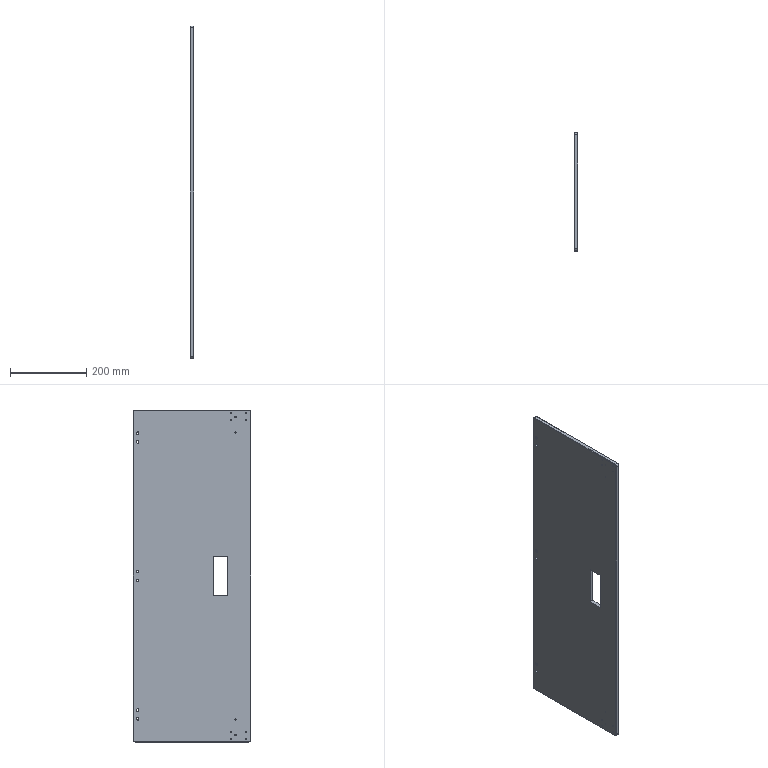Part | NX | 1 solid | 48 faces | box 10 x 308 x 869 mm | volume 2633126 mm3 | cylinder 22 | plane 18 | cone 8 | commonest cylinder face diameters 2.5 x8 6.5 x6 3.3 x4 10 x4
STEP:
#1=CARTESIAN_POINT('',(10.,-268.,-377.35));
#2=VERTEX_POINT('',#1);
#3=CARTESIAN_POINT('',(10.,-268.,-375.7));
#4=DIRECTION('',(1.,0.,0.));
#5=DIRECTION('',(0.,0.,-1.));
#6=AXIS2_PLACEMENT_3D('',#3,#4,#5);
#7=CIRCLE('',#6,1.65);
#8=EDGE_CURVE('',#2,#2,#7,.T.);
#9=ORIENTED_EDGE('',*,*,#8,.F.);
#10=EDGE_LOOP('',(#9));
#11=FACE_BOUND('',#10,.T.);
#12=CARTESIAN_POINT('',(10.,-268.,414.05));
#13=VERTEX_POINT('',#12);
#14=CARTESIAN_POINT('',(10.,-268.,415.7));
#15=DIRECTION('',(1.,0.,0.));
#16=DIRECTION('',(0.,0.,-1.));
#17=AXIS2_PLACEMENT_3D('',#14,#15,#16);
#18=CIRCLE('',#17,1.65);
#19=EDGE_CURVE('',#13,#13,#18,.T.);
#20=ORIENTED_EDGE('',*,*,#19,.F.);
#21=EDGE_LOOP('',(#20));
#22=FACE_BOUND('',#21,.T.);
#23=CARTESIAN_POINT('',(10.,-268.,374.05));
#24=VERTEX_POINT('',#23);
#25=CARTESIAN_POINT('',(10.,-268.,375.7));
#26=DIRECTION('',(1.,0.,0.));
#27=DIRECTION('',(0.,0.,-1.));
#28=AXIS2_PLACEMENT_3D('',#25,#26,#27);
#29=CIRCLE('',#28,1.65);
#30=EDGE_CURVE('',#24,#24,#29,.T.);
#31=ORIENTED_EDGE('',*,*,#30,.F.);
#32=EDGE_LOOP('',(#31));
#33=FACE_BOUND('',#32,.T.);
#34=CARTESIAN_POINT('',(10.,-256.,407.25));
#35=VERTEX_POINT('',#34);
#36=CARTESIAN_POINT('',(10.,-256.,408.5));
#37=DIRECTION('',(1.,0.,0.));
#38=DIRECTION('',(0.,0.,-1.));
#39=AXIS2_PLACEMENT_3D('',#36,#37,#38);
#40=CIRCLE('',#39,1.25);
#41=EDGE_CURVE('',#35,#35,#40,.T.);
#42=ORIENTED_EDGE('',*,*,#41,.F.);
#43=EDGE_LOOP('',(#42));
#44=FACE_BOUND('',#43,.T.);
#45=CARTESIAN_POINT('',(10.,-296.,407.25));
#46=VERTEX_POINT('',#45);
#47=CARTESIAN_POINT('',(10.,-296.,408.5));
#48=DIRECTION('',(1.,0.,0.));
#49=DIRECTION('',(0.,0.,-1.));
#50=AXIS2_PLACEMENT_3D('',#47,#48,#49);
#51=CIRCLE('',#50,1.25);
#52=EDGE_CURVE('',#46,#46,#51,.T.);
#53=ORIENTED_EDGE('',*,*,#52,.F.);
#54=EDGE_LOOP('',(#53));
#55=FACE_BOUND('',#54,.T.);
#56=CARTESIAN_POINT('',(10.,-296.,425.25));
#57=VERTEX_POINT('',#56);
#58=CARTESIAN_POINT('',(10.,-296.,426.5));
#59=DIRECTION('',(1.,0.,0.));
#60=DIRECTION('',(0.,0.,-1.));
#61=AXIS2_PLACEMENT_3D('',#58,#59,#60);
#62=CIRCLE('',#61,1.25);
#63=EDGE_CURVE('',#57,#57,#62,.T.);
#64=ORIENTED_EDGE('',*,*,#63,.F.);
#65=EDGE_LOOP('',(#64));
#66=FACE_BOUND('',#65,.T.);
#67=CARTESIAN_POINT('',(10.,-256.,425.25));
#68=VERTEX_POINT('',#67);
#69=CARTESIAN_POINT('',(10.,-256.,426.5));
#70=DIRECTION('',(1.,0.,0.));
#71=DIRECTION('',(0.,0.,-1.));
#72=AXIS2_PLACEMENT_3D('',#69,#70,#71);
#73=CIRCLE('',#72,1.25);
#74=EDGE_CURVE('',#68,#68,#73,.T.);
#75=ORIENTED_EDGE('',*,*,#74,.F.);
#76=EDGE_LOOP('',(#75));
#77=FACE_BOUND('',#76,.T.);
#78=CARTESIAN_POINT('',(10.,-256.,-427.75));
#79=VERTEX_POINT('',#78);
#80=CARTESIAN_POINT('',(10.,-256.,-426.5));
#81=DIRECTION('',(1.,0.,0.));
#82=DIRECTION('',(0.,0.,-1.));
#83=AXIS2_PLACEMENT_3D('',#80,#81,#82);
#84=CIRCLE('',#83,1.25);
#85=EDGE_CURVE('',#79,#79,#84,.T.);
#86=ORIENTED_EDGE('',*,*,#85,.F.);
#87=EDGE_LOOP('',(#86));
#88=FACE_BOUND('',#87,.T.);
#89=CARTESIAN_POINT('',(10.,-296.,-427.75));
#90=VERTEX_POINT('',#89);
#91=CARTESIAN_POINT('',(10.,-296.,-426.5));
#92=DIRECTION('',(1.,0.,0.));
#93=DIRECTION('',(0.,0.,-1.));
#94=AXIS2_PLACEMENT_3D('',#91,#92,#93);
#95=CIRCLE('',#94,1.25);
#96=EDGE_CURVE('',#90,#90,#95,.T.);
#97=ORIENTED_EDGE('',*,*,#96,.F.);
#98=EDGE_LOOP('',(#97));
#99=FACE_BOUND('',#98,.T.);
#100=CARTESIAN_POINT('',(10.,-296.,-409.75));
#101=VERTEX_POINT('',#100);
#102=CARTESIAN_POINT('',(10.,-296.,-408.5));
#103=DIRECTION('',(1.,0.,0.));
#104=DIRECTION('',(0.,0.,-1.));
#105=AXIS2_PLACEMENT_3D('',#102,#103,#104);
#106=CIRCLE('',#105,1.25);
#107=EDGE_CURVE('',#101,#101,#106,.T.);
#108=ORIENTED_EDGE('',*,*,#107,.F.);
#109=EDGE_LOOP('',(#108));
#110=FACE_BOUND('',#109,.T.);
#111=CARTESIAN_POINT('',(10.,-256.,-409.75));
#112=VERTEX_POINT('',#111);
#113=CARTESIAN_POINT('',(10.,-256.,-408.5));
#114=DIRECTION('',(1.,0.,0.));
#115=DIRECTION('',(0.,0.,-1.));
#116=AXIS2_PLACEMENT_3D('',#113,#114,#115);
#117=CIRCLE('',#116,1.25);
#118=EDGE_CURVE('',#112,#112,#117,.T.);
#119=ORIENTED_EDGE('',*,*,#118,.F.);
#120=EDGE_LOOP('',(#119));
#121=FACE_BOUND('',#120,.T.);
#122=CARTESIAN_POINT('',(10.,-5.,-433.5));
#123=VERTEX_POINT('',#122);
#124=CARTESIAN_POINT('',(10.,-1.,-429.5));
#125=VERTEX_POINT('',#124);
#126=CARTESIAN_POINT('',(10.,-5.,-429.5));
#127=DIRECTION('',(-1.,0.,0.));
#128=DIRECTION('',(0.,-1.,0.));
#129=AXIS2_PLACEMENT_3D('',#126,#127,#128);
#130=CIRCLE('',#129,4.);
#131=EDGE_CURVE('',#123,#125,#130,.F.);
#132=ORIENTED_EDGE('',*,*,#131,.T.);
#133=CARTESIAN_POINT('',(10.,-1.,429.5));
#134=VERTEX_POINT('',#133);
#135=CARTESIAN_POINT('',(10.,-1.,434.5));
#136=DIRECTION('',(0.,0.,1.));
#137=VECTOR('',#136,1000.);
#138=LINE('',#135,#137);
#139=EDGE_CURVE('',#125,#134,#138,.T.);
#140=ORIENTED_EDGE('',*,*,#139,.T.);
#141=CARTESIAN_POINT('',(10.,-5.,433.5));
#142=VERTEX_POINT('',#141);
#143=CARTESIAN_POINT('',(10.,-5.,429.5));
#144=DIRECTION('',(-1.,0.,0.));
#145=DIRECTION('',(0.,-1.,0.));
#146=AXIS2_PLACEMENT_3D('',#143,#144,#145);
#147=CIRCLE('',#146,4.);
#148=EDGE_CURVE('',#134,#142,#147,.F.);
#149=ORIENTED_EDGE('',*,*,#148,.T.);
#150=CARTESIAN_POINT('',(10.,-303.,433.5));
#151=VERTEX_POINT('',#150);
#152=CARTESIAN_POINT('',(10.,0.,433.5));
#153=DIRECTION('',(0.,-1.,0.));
#154=VECTOR('',#153,1000.);
#155=LINE('',#152,#154);
#156=EDGE_CURVE('',#142,#151,#155,.T.);
#157=ORIENTED_EDGE('',*,*,#156,.T.);
#158=CARTESIAN_POINT('',(10.,-307.,429.5));
#159=VERTEX_POINT('',#158);
#160=CARTESIAN_POINT('',(10.,-303.,429.5));
#161=DIRECTION('',(-1.,0.,0.));
#162=DIRECTION('',(0.,-1.,0.));
#163=AXIS2_PLACEMENT_3D('',#160,#161,#162);
#164=CIRCLE('',#163,4.);
#165=EDGE_CURVE('',#151,#159,#164,.F.);
#166=ORIENTED_EDGE('',*,*,#165,.T.);
#167=CARTESIAN_POINT('',(10.,-307.,-429.5));
#168=VERTEX_POINT('',#167);
#169=CARTESIAN_POINT('',(10.,-307.,434.5));
#170=DIRECTION('',(0.,0.,-1.));
#171=VECTOR('',#170,1000.);
#172=LINE('',#169,#171);
#173=EDGE_CURVE('',#159,#168,#172,.T.);
#174=ORIENTED_EDGE('',*,*,#173,.T.);
#175=CARTESIAN_POINT('',(10.,-303.,-433.5));
#176=VERTEX_POINT('',#175);
#177=CARTESIAN_POINT('',(10.,-303.,-429.5));
#178=DIRECTION('',(-1.,0.,0.));
#179=DIRECTION('',(0.,-1.,0.));
#180=AXIS2_PLACEMENT_3D('',#177,#178,#179);
#181=CIRCLE('',#180,4.);
#182=EDGE_CURVE('',#168,#176,#181,.F.);
#183=ORIENTED_EDGE('',*,*,#182,.T.);
#184=CARTESIAN_POINT('',(10.,-5.,-433.5));
#185=DIRECTION('',(0.,1.,0.));
#186=VECTOR('',#185,1000.);
#187=LINE('',#184,#186);
#188=EDGE_CURVE('',#176,#123,#187,.T.);
#189=ORIENTED_EDGE('',*,*,#188,.T.);
#190=EDGE_LOOP('',(#132,#140,#149,#157,#166,#174,#183,#189));
#191=FACE_BOUND('',#190,.T.);
#192=CARTESIAN_POINT('',(10.,-12.,-377.25));
#193=VERTEX_POINT('',#192);
#194=CARTESIAN_POINT('',(10.,-12.,-374.));
#195=DIRECTION('',(1.,0.,0.));
#196=DIRECTION('',(0.,0.,-1.));
#197=AXIS2_PLACEMENT_3D('',#194,#195,#196);
#198=CIRCLE('',#197,3.25);
#199=EDGE_CURVE('',#193,#193,#198,.T.);
#200=ORIENTED_EDGE('',*,*,#199,.F.);
#201=EDGE_LOOP('',(#200));
#202=FACE_BOUND('',#201,.T.);
#203=CARTESIAN_POINT('',(10.,-12.,-354.25));
#204=VERTEX_POINT('',#203);
#205=CARTESIAN_POINT('',(10.,-12.,-351.));
#206=DIRECTION('',(1.,0.,0.));
#207=DIRECTION('',(0.,0.,-1.));
#208=AXIS2_PLACEMENT_3D('',#205,#206,#207);
#209=CIRCLE('',#208,3.25);
#210=EDGE_CURVE('',#204,#204,#209,.T.);
#211=ORIENTED_EDGE('',*,*,#210,.F.);
#212=EDGE_LOOP('',(#211));
#213=FACE_BOUND('',#212,.T.);
#214=CARTESIAN_POINT('',(10.,-12.,347.75));
#215=VERTEX_POINT('',#214);
#216=CARTESIAN_POINT('',(10.,-12.,351.));
#217=DIRECTION('',(1.,0.,0.));
#218=DIRECTION('',(0.,0.,-1.));
#219=AXIS2_PLACEMENT_3D('',#216,#217,#218);
#220=CIRCLE('',#219,3.25);
#221=EDGE_CURVE('',#215,#215,#220,.T.);
#222=ORIENTED_EDGE('',*,*,#221,.F.);
#223=EDGE_LOOP('',(#222));
#224=FACE_BOUND('',#223,.T.);
#225=CARTESIAN_POINT('',(10.,-12.,370.75));
#226=VERTEX_POINT('',#225);
#227=CARTESIAN_POINT('',(10.,-12.,374.));
#228=DIRECTION('',(1.,0.,0.));
#229=DIRECTION('',(0.,0.,-1.));
#230=AXIS2_PLACEMENT_3D('',#227,#228,#229);
#231=CIRCLE('',#230,3.25);
#232=EDGE_CURVE('',#226,#226,#231,.T.);
#233=ORIENTED_EDGE('',*,*,#232,.F.);
#234=EDGE_LOOP('',(#233));
#235=FACE_BOUND('',#234,.T.);
#236=CARTESIAN_POINT('',(10.,-12.,8.25));
#237=VERTEX_POINT('',#236);
#238=CARTESIAN_POINT('',(10.,-12.,11.5));
#239=DIRECTION('',(1.,0.,0.));
#240=DIRECTION('',(0.,0.,-1.));
#241=AXIS2_PLACEMENT_3D('',#238,#239,#240);
#242=CIRCLE('',#241,3.25);
#243=EDGE_CURVE('',#237,#237,#242,.T.);
#244=ORIENTED_EDGE('',*,*,#243,.F.);
#245=EDGE_LOOP('',(#244));
#246=FACE_BOUND('',#245,.T.);
#247=CARTESIAN_POINT('',(10.,-12.,-14.75));
#248=VERTEX_POINT('',#247);
#249=CARTESIAN_POINT('',(10.,-12.,-11.5));
#250=DIRECTION('',(1.,0.,0.));
#251=DIRECTION('',(0.,0.,-1.));
#252=AXIS2_PLACEMENT_3D('',#249,#250,#251);
#253=CIRCLE('',#252,3.25);
#254=EDGE_CURVE('',#248,#248,#253,.T.);
#255=ORIENTED_EDGE('',*,*,#254,.F.);
#256=EDGE_LOOP('',(#255));
#257=FACE_BOUND('',#256,.T.);
#258=CARTESIAN_POINT('',(10.,-211.,-51.5));
#259=VERTEX_POINT('',#258);
#260=CARTESIAN_POINT('',(10.,-211.,51.5));
#261=VERTEX_POINT('',#260);
#262=CARTESIAN_POINT('',(10.,-211.,51.5));
#263=DIRECTION('',(0.,0.,1.));
#264=VECTOR('',#263,1000.);
#265=LINE('',#262,#264);
#266=EDGE_CURVE('',#259,#261,#265,.T.);
#267=ORIENTED_EDGE('',*,*,#266,.F.);
#268=CARTESIAN_POINT('',(10.,-248.,-51.5));
#269=VERTEX_POINT('',#268);
#270=CARTESIAN_POINT('',(10.,-211.,-51.5));
#271=DIRECTION('',(0.,1.,0.));
#272=VECTOR('',#271,1000.);
#273=LINE('',#270,#272);
#274=EDGE_CURVE('',#269,#259,#273,.T.);
#275=ORIENTED_EDGE('',*,*,#274,.F.);
#276=CARTESIAN_POINT('',(10.,-248.,51.5));
#277=VERTEX_POINT('',#276);
#278=CARTESIAN_POINT('',(10.,-248.,51.5));
#279=DIRECTION('',(0.,0.,-1.));
#280=VECTOR('',#279,1000.);
#281=LINE('',#278,#280);
#282=EDGE_CURVE('',#277,#269,#281,.T.);
#283=ORIENTED_EDGE('',*,*,#282,.F.);
#284=CARTESIAN_POINT('',(10.,-211.,51.5));
#285=DIRECTION('',(0.,-1.,0.));
#286=VECTOR('',#285,1000.);
#287=LINE('',#284,#286);
#288=EDGE_CURVE('',#261,#277,#287,.T.);
#289=ORIENTED_EDGE('',*,*,#288,.F.);
#290=EDGE_LOOP('',(#267,#275,#283,#289));
#291=FACE_BOUND('',#290,.T.);
#292=CARTESIAN_POINT('',(10.,-268.,-417.35));
#293=VERTEX_POINT('',#292);
#294=CARTESIAN_POINT('',(10.,-268.,-415.7));
#295=DIRECTION('',(1.,0.,0.));
#296=DIRECTION('',(0.,0.,-1.));
#297=AXIS2_PLACEMENT_3D('',#294,#295,#296);
#298=CIRCLE('',#297,1.65);
#299=EDGE_CURVE('',#293,#293,#298,.T.);
#300=ORIENTED_EDGE('',*,*,#299,.F.);
#301=EDGE_LOOP('',(#300));
#302=FACE_BOUND('',#301,.T.);
#303=CARTESIAN_POINT('',(10.,0.,434.5));
#304=DIRECTION('',(-1.,0.,0.));
#305=DIRECTION('',(0.,-1.,0.));
#306=AXIS2_PLACEMENT_3D('',#303,#304,#305);
#307=PLANE('',#306);
#308=ADVANCED_FACE('',(#11,#22,#33,#44,#55,#66,#77,#88,#99,#110,#121,#191,#202,#213,#224,#235,#246,#257,#291,#302),#307,.F.);
#309=CARTESIAN_POINT('',(0.,-268.,-417.35));
#310=VERTEX_POINT('',#309);
#311=CARTESIAN_POINT('',(0.,-268.,-415.7));
#312=DIRECTION('',(1.,0.,0.));
#313=DIRECTION('',(0.,0.,-1.));
#314=AXIS2_PLACEMENT_3D('',#311,#312,#313);
#315=CIRCLE('',#314,1.65);
#316=EDGE_CURVE('',#310,#310,#315,.T.);
#317=ORIENTED_EDGE('',*,*,#316,.T.);
#318=EDGE_LOOP('',(#317));
#319=FACE_BOUND('',#318,.T.);
#320=CARTESIAN_POINT('',(0.,-268.,-377.35));
#321=VERTEX_POINT('',#320);
#322=CARTESIAN_POINT('',(0.,-268.,-375.7));
#323=DIRECTION('',(1.,0.,0.));
#324=DIRECTION('',(0.,0.,-1.));
#325=AXIS2_PLACEMENT_3D('',#322,#323,#324);
#326=CIRCLE('',#325,1.65);
#327=EDGE_CURVE('',#321,#321,#326,.T.);
#328=ORIENTED_EDGE('',*,*,#327,.T.);
#329=EDGE_LOOP('',(#328));
#330=FACE_BOUND('',#329,.T.);
#331=CARTESIAN_POINT('',(0.,-268.,414.05));
#332=VERTEX_POINT('',#331);
#333=CARTESIAN_POINT('',(0.,-268.,415.7));
#334=DIRECTION('',(1.,0.,0.));
#335=DIRECTION('',(0.,0.,-1.));
#336=AXIS2_PLACEMENT_3D('',#333,#334,#335);
#337=CIRCLE('',#336,1.65);
#338=EDGE_CURVE('',#332,#332,#337,.T.);
#339=ORIENTED_EDGE('',*,*,#338,.T.);
#340=EDGE_LOOP('',(#339));
#341=FACE_BOUND('',#340,.T.);
#342=CARTESIAN_POINT('',(0.,-268.,374.05));
#343=VERTEX_POINT('',#342);
#344=CARTESIAN_POINT('',(0.,-268.,375.7));
#345=DIRECTION('',(1.,0.,0.));
#346=DIRECTION('',(0.,0.,-1.));
#347=AXIS2_PLACEMENT_3D('',#344,#345,#346);
#348=CIRCLE('',#347,1.65);
#349=EDGE_CURVE('',#343,#343,#348,.T.);
#350=ORIENTED_EDGE('',*,*,#349,.T.);
#351=EDGE_LOOP('',(#350));
#352=FACE_BOUND('',#351,.T.);
#353=CARTESIAN_POINT('',(0.,-256.,407.25));
#354=VERTEX_POINT('',#353);
#355=CARTESIAN_POINT('',(0.,-256.,408.5));
#356=DIRECTION('',(1.,0.,0.));
#357=DIRECTION('',(0.,0.,-1.));
#358=AXIS2_PLACEMENT_3D('',#355,#356,#357);
#359=CIRCLE('',#358,1.25);
#360=EDGE_CURVE('',#354,#354,#359,.T.);
#361=ORIENTED_EDGE('',*,*,#360,.T.);
#362=EDGE_LOOP('',(#361));
#363=FACE_BOUND('',#362,.T.);
#364=CARTESIAN_POINT('',(0.,-296.,407.25));
#365=VERTEX_POINT('',#364);
#366=CARTESIAN_POINT('',(0.,-296.,408.5));
#367=DIRECTION('',(1.,0.,0.));
#368=DIRECTION('',(0.,0.,-1.));
#369=AXIS2_PLACEMENT_3D('',#366,#367,#368);
#370=CIRCLE('',#369,1.25);
#371=EDGE_CURVE('',#365,#365,#370,.T.);
#372=ORIENTED_EDGE('',*,*,#371,.T.);
#373=EDGE_LOOP('',(#372));
#374=FACE_BOUND('',#373,.T.);
#375=CARTESIAN_POINT('',(0.,-296.,425.25));
#376=VERTEX_POINT('',#375);
#377=CARTESIAN_POINT('',(0.,-296.,426.5));
#378=DIRECTION('',(1.,0.,0.));
#379=DIRECTION('',(0.,0.,-1.));
#380=AXIS2_PLACEMENT_3D('',#377,#378,#379);
#381=CIRCLE('',#380,1.25);
#382=EDGE_CURVE('',#376,#376,#381,.T.);
#383=ORIENTED_EDGE('',*,*,#382,.T.);
#384=EDGE_LOOP('',(#383));
#385=FACE_BOUND('',#384,.T.);
#386=CARTESIAN_POINT('',(0.,-256.,425.25));
#387=VERTEX_POINT('',#386);
#388=CARTESIAN_POINT('',(0.,-256.,426.5));
#389=DIRECTION('',(1.,0.,0.));
#390=DIRECTION('',(0.,0.,-1.));
#391=AXIS2_PLACEMENT_3D('',#388,#389,#390);
#392=CIRCLE('',#391,1.25);
#393=EDGE_CURVE('',#387,#387,#392,.T.);
#394=ORIENTED_EDGE('',*,*,#393,.T.);
#395=EDGE_LOOP('',(#394));
#396=FACE_BOUND('',#395,.T.);
#397=CARTESIAN_POINT('',(0.,-256.,-427.75));
#398=VERTEX_POINT('',#397);
#399=CARTESIAN_POINT('',(0.,-256.,-426.5));
#400=DIRECTION('',(1.,0.,0.));
#401=DIRECTION('',(0.,0.,-1.));
#402=AXIS2_PLACEMENT_3D('',#399,#400,#401);
#403=CIRCLE('',#402,1.25);
#404=EDGE_CURVE('',#398,#398,#403,.T.);
#405=ORIENTED_EDGE('',*,*,#404,.T.);
#406=EDGE_LOOP('',(#405));
#407=FACE_BOUND('',#406,.T.);
#408=CARTESIAN_POINT('',(0.,-296.,-427.75));
#409=VERTEX_POINT('',#408);
#410=CARTESIAN_POINT('',(0.,-296.,-426.5));
#411=DIRECTION('',(1.,0.,0.));
#412=DIRECTION('',(0.,0.,-1.));
#413=AXIS2_PLACEMENT_3D('',#410,#411,#412);
#414=CIRCLE('',#413,1.25);
#415=EDGE_CURVE('',#409,#409,#414,.T.);
#416=ORIENTED_EDGE('',*,*,#415,.T.);
#417=EDGE_LOOP('',(#416));
#418=FACE_BOUND('',#417,.T.);
#419=CARTESIAN_POINT('',(0.,-296.,-409.75));
#420=VERTEX_POINT('',#419);
#421=CARTESIAN_POINT('',(0.,-296.,-408.5));
#422=DIRECTION('',(1.,0.,0.));
#423=DIRECTION('',(0.,0.,-1.));
#424=AXIS2_PLACEMENT_3D('',#421,#422,#423);
#425=CIRCLE('',#424,1.25);
#426=EDGE_CURVE('',#420,#420,#425,.T.);
#427=ORIENTED_EDGE('',*,*,#426,.T.);
#428=EDGE_LOOP('',(#427));
#429=FACE_BOUND('',#428,.T.);
#430=CARTESIAN_POINT('',(0.,-256.,-409.75));
#431=VERTEX_POINT('',#430);
#432=CARTESIAN_POINT('',(0.,-256.,-408.5));
#433=DIRECTION('',(1.,0.,0.));
#434=DIRECTION('',(0.,0.,-1.));
#435=AXIS2_PLACEMENT_3D('',#432,#433,#434);
#436=CIRCLE('',#435,1.25);
#437=EDGE_CURVE('',#431,#431,#436,.T.);
#438=ORIENTED_EDGE('',*,*,#437,.T.);
#439=EDGE_LOOP('',(#438));
#440=FACE_BOUND('',#439,.T.);
#441=CARTESIAN_POINT('',(0.,-5.,433.5));
#442=VERTEX_POINT('',#441);
#443=CARTESIAN_POINT('',(0.,-1.,429.5));
#444=VERTEX_POINT('',#443);
#445=CARTESIAN_POINT('',(0.,-5.,429.5));
#446=DIRECTION('',(1.,0.,0.));
#447=DIRECTION('',(0.,0.,-1.));
#448=AXIS2_PLACEMENT_3D('',#445,#446,#447);
#449=CIRCLE('',#448,4.);
#450=EDGE_CURVE('',#442,#444,#449,.F.);
#451=ORIENTED_EDGE('',*,*,#450,.T.);
#452=CARTESIAN_POINT('',(0.,-1.,-429.5));
#453=VERTEX_POINT('',#452);
#454=CARTESIAN_POINT('',(0.,-1.,434.5));
#455=DIRECTION('',(0.,0.,-1.));
#456=VECTOR('',#455,1000.);
#457=LINE('',#454,#456);
#458=EDGE_CURVE('',#444,#453,#457,.T.);
#459=ORIENTED_EDGE('',*,*,#458,.T.);
#460=CARTESIAN_POINT('',(0.,-5.,-433.5));
#461=VERTEX_POINT('',#460);
#462=CARTESIAN_POINT('',(0.,-5.,-429.5));
#463=DIRECTION('',(1.,0.,0.));
#464=DIRECTION('',(0.,0.,-1.));
#465=AXIS2_PLACEMENT_3D('',#462,#463,#464);
#466=CIRCLE('',#465,4.);
#467=EDGE_CURVE('',#453,#461,#466,.F.);
#468=ORIENTED_EDGE('',*,*,#467,.T.);
#469=CARTESIAN_POINT('',(0.,-303.,-433.5));
#470=VERTEX_POINT('',#469);
#471=CARTESIAN_POINT('',(0.,-303.,-433.5));
#472=DIRECTION('',(0.,-1.,0.));
#473=VECTOR('',#472,1000.);
#474=LINE('',#471,#473);
#475=EDGE_CURVE('',#461,#470,#474,.T.);
#476=ORIENTED_EDGE('',*,*,#475,.T.);
#477=CARTESIAN_POINT('',(0.,-307.,-429.5));
#478=VERTEX_POINT('',#477);
#479=CARTESIAN_POINT('',(0.,-303.,-429.5));
#480=DIRECTION('',(1.,0.,0.));
#481=DIRECTION('',(0.,0.,-1.));
#482=AXIS2_PLACEMENT_3D('',#479,#480,#481);
#483=CIRCLE('',#482,4.);
#484=EDGE_CURVE('',#470,#478,#483,.F.);
#485=ORIENTED_EDGE('',*,*,#484,.T.);
#486=CARTESIAN_POINT('',(0.,-307.,429.5));
#487=VERTEX_POINT('',#486);
#488=CARTESIAN_POINT('',(0.,-307.,434.5));
#489=DIRECTION('',(0.,0.,1.));
#490=VECTOR('',#489,1000.);
#491=LINE('',#488,#490);
#492=EDGE_CURVE('',#478,#487,#491,.T.);
#493=ORIENTED_EDGE('',*,*,#492,.T.);
#494=CARTESIAN_POINT('',(0.,-303.,433.5));
#495=VERTEX_POINT('',#494);
#496=CARTESIAN_POINT('',(0.,-303.,429.5));
#497=DIRECTION('',(1.,0.,0.));
#498=DIRECTION('',(0.,0.,-1.));
#499=AXIS2_PLACEMENT_3D('',#496,#497,#498);
#500=CIRCLE('',#499,4.);
#501=EDGE_CURVE('',#487,#495,#500,.F.);
#502=ORIENTED_EDGE('',*,*,#501,.T.);
#503=CARTESIAN_POINT('',(0.,-308.,433.5));
#504=DIRECTION('',(0.,1.,0.));
#505=VECTOR('',#504,1000.);
#506=LINE('',#503,#505);
#507=EDGE_CURVE('',#495,#442,#506,.T.);
#508=ORIENTED_EDGE('',*,*,#507,.T.);
#509=EDGE_LOOP('',(#451,#459,#468,#476,#485,#493,#502,#508));
#510=FACE_BOUND('',#509,.T.);
#511=CARTESIAN_POINT('',(0.,-12.,-377.25));
#512=VERTEX_POINT('',#511);
#513=CARTESIAN_POINT('',(0.,-12.,-374.));
#514=DIRECTION('',(1.,0.,0.));
#515=DIRECTION('',(0.,0.,-1.));
#516=AXIS2_PLACEMENT_3D('',#513,#514,#515);
#517=CIRCLE('',#516,3.25);
#518=EDGE_CURVE('',#512,#512,#517,.T.);
#519=ORIENTED_EDGE('',*,*,#518,.T.);
#520=EDGE_LOOP('',(#519));
#521=FACE_BOUND('',#520,.T.);
#522=CARTESIAN_POINT('',(0.,-12.,-354.25));
#523=VERTEX_POINT('',#522);
#524=CARTESIAN_POINT('',(0.,-12.,-351.));
#525=DIRECTION('',(1.,0.,0.));
#526=DIRECTION('',(0.,0.,-1.));
#527=AXIS2_PLACEMENT_3D('',#524,#525,#526);
#528=CIRCLE('',#527,3.25);
#529=EDGE_CURVE('',#523,#523,#528,.T.);
#530=ORIENTED_EDGE('',*,*,#529,.T.);
#531=EDGE_LOOP('',(#530));
#532=FACE_BOUND('',#531,.T.);
#533=CARTESIAN_POINT('',(0.,-12.,347.75));
#534=VERTEX_POINT('',#533);
#535=CARTESIAN_POINT('',(0.,-12.,351.));
#536=DIRECTION('',(1.,0.,0.));
#537=DIRECTION('',(0.,0.,-1.));
#538=AXIS2_PLACEMENT_3D('',#535,#536,#537);
#539=CIRCLE('',#538,3.25);
#540=EDGE_CURVE('',#534,#534,#539,.T.);
#541=ORIENTED_EDGE('',*,*,#540,.T.);
#542=EDGE_LOOP('',(#541));
#543=FACE_BOUND('',#542,.T.);
#544=CARTESIAN_POINT('',(0.,-12.,370.75));
#545=VERTEX_POINT('',#544);
#546=CARTESIAN_POINT('',(0.,-12.,374.));
#547=DIRECTION('',(1.,0.,0.));
#548=DIRECTION('',(0.,0.,-1.));
#549=AXIS2_PLACEMENT_3D('',#546,#547,#548);
#550=CIRCLE('',#549,3.25);
#551=EDGE_CURVE('',#545,#545,#550,.T.);
#552=ORIENTED_EDGE('',*,*,#551,.T.);
#553=EDGE_LOOP('',(#552));
#554=FACE_BOUND('',#553,.T.);
#555=CARTESIAN_POINT('',(0.,-12.,8.25));
#556=VERTEX_POINT('',#555);
#557=CARTESIAN_POINT('',(0.,-12.,11.5));
#558=DIRECTION('',(1.,0.,0.));
#559=DIRECTION('',(0.,0.,-1.));
#560=AXIS2_PLACEMENT_3D('',#557,#558,#559);
#561=CIRCLE('',#560,3.25);
#562=EDGE_CURVE('',#556,#556,#561,.T.);
#563=ORIENTED_EDGE('',*,*,#562,.T.);
#564=EDGE_LOOP('',(#563));
#565=FACE_BOUND('',#564,.T.);
#566=CARTESIAN_POINT('',(0.,-12.,-14.75));
#567=VERTEX_POINT('',#566);
#568=CARTESIAN_POINT('',(0.,-12.,-11.5));
#569=DIRECTION('',(1.,0.,0.));
#570=DIRECTION('',(0.,0.,-1.));
#571=AXIS2_PLACEMENT_3D('',#568,#569,#570);
#572=CIRCLE('',#571,3.25);
#573=EDGE_CURVE('',#567,#567,#572,.T.);
#574=ORIENTED_EDGE('',*,*,#573,.T.);
#575=EDGE_LOOP('',(#574));
#576=FACE_BOUND('',#575,.T.);
#577=CARTESIAN_POINT('',(0.,-248.,51.5));
#578=VERTEX_POINT('',#577);
#579=CARTESIAN_POINT('',(0.,-248.,-51.5));
#580=VERTEX_POINT('',#579);
#581=CARTESIAN_POINT('',(0.,-248.,51.5));
#582=DIRECTION('',(0.,0.,-1.));
#583=VECTOR('',#582,1000.);
#584=LINE('',#581,#583);
#585=EDGE_CURVE('',#578,#580,#584,.T.);
#586=ORIENTED_EDGE('',*,*,#585,.T.);
#587=CARTESIAN_POINT('',(0.,-211.,-51.5));
#588=VERTEX_POINT('',#587);
#589=CARTESIAN_POINT('',(0.,-211.,-51.5));
#590=DIRECTION('',(0.,1.,0.));
#591=VECTOR('',#590,1000.);
#592=LINE('',#589,#591);
#593=EDGE_CURVE('',#580,#588,#592,.T.);
#594=ORIENTED_EDGE('',*,*,#593,.T.);
#595=CARTESIAN_POINT('',(0.,-211.,51.5));
#596=VERTEX_POINT('',#595);
#597=CARTESIAN_POINT('',(0.,-211.,51.5));
#598=DIRECTION('',(0.,0.,1.));
#599=VECTOR('',#598,1000.);
#600=LINE('',#597,#599);
#601=EDGE_CURVE('',#588,#596,#600,.T.);
#602=ORIENTED_EDGE('',*,*,#601,.T.);
#603=CARTESIAN_POINT('',(0.,-211.,51.5));
#604=DIRECTION('',(0.,-1.,0.));
#605=VECTOR('',#604,1000.);
#606=LINE('',#603,#605);
#607=EDGE_CURVE('',#596,#578,#606,.T.);
#608=ORIENTED_EDGE('',*,*,#607,.T.);
#609=EDGE_LOOP('',(#586,#594,#602,#608));
#610=FACE_BOUND('',#609,.T.);
#611=CARTESIAN_POINT('',(0.,-308.,434.5));
#612=DIRECTION('',(1.,0.,0.));
#613=DIRECTION('',(0.,0.,-1.));
#614=AXIS2_PLACEMENT_3D('',#611,#612,#613);
#615=PLANE('',#614);
#616=ADVANCED_FACE('',(#319,#330,#341,#352,#363,#374,#385,#396,#407,#418,#429,#440,#510,#521,#532,#543,#554,#565,#576,#610),#615,.F.);
#617=CARTESIAN_POINT('',(1.,-308.,-429.5));
#618=VERTEX_POINT('',#617);
#619=CARTESIAN_POINT('',(9.,-308.,-429.5));
#620=VERTEX_POINT('',#619);
#621=CARTESIAN_POINT('',(10.,-308.,-429.5));
#622=DIRECTION('',(1.,0.,0.));
#623=VECTOR('',#622,1000.);
#624=LINE('',#621,#623);
#625=EDGE_CURVE('',#618,#620,#624,.T.);
#626=ORIENTED_EDGE('',*,*,#625,.T.);
#627=CARTESIAN_POINT('',(9.,-308.,429.5));
#628=VERTEX_POINT('',#627);
#629=CARTESIAN_POINT('',(9.,-308.,434.5));
#630=DIRECTION('',(0.,0.,1.));
#631=VECTOR('',#630,1000.);
#632=LINE('',#629,#631);
#633=EDGE_CURVE('',#620,#628,#632,.T.);
#634=ORIENTED_EDGE('',*,*,#633,.T.);
#635=CARTESIAN_POINT('',(1.,-308.,429.5));
#636=VERTEX_POINT('',#635);
#637=CARTESIAN_POINT('',(10.,-308.,429.5));
#638=DIRECTION('',(1.,0.,0.));
#639=VECTOR('',#638,1000.);
#640=LINE('',#637,#639);
#641=EDGE_CURVE('',#628,#636,#640,.F.);
#642=ORIENTED_EDGE('',*,*,#641,.T.);
#643=CARTESIAN_POINT('',(1.,-308.,434.5));
#644=DIRECTION('',(0.,0.,-1.));
#645=VECTOR('',#644,1000.);
#646=LINE('',#643,#645);
#647=EDGE_CURVE('',#636,#618,#646,.T.);
#648=ORIENTED_EDGE('',*,*,#647,.T.);
#649=EDGE_LOOP('',(#626,#634,#642,#648));
#650=FACE_BOUND('',#649,.T.);
#651=CARTESIAN_POINT('',(10.,-308.,434.5));
#652=DIRECTION('',(0.,1.,0.));
#653=DIRECTION('',(0.,0.,1.));
#654=AXIS2_PLACEMENT_3D('',#651,#652,#653);
#655=PLANE('',#654);
#656=ADVANCED_FACE('',(#650),#655,.F.);
#657=CARTESIAN_POINT('',(1.,0.,429.5));
#658=VERTEX_POINT('',#657);
#659=CARTESIAN_POINT('',(9.,0.,429.5));
#660=VERTEX_POINT('',#659);
#661=CARTESIAN_POINT('',(0.,0.,429.5));
#662=DIRECTION('',(-1.,0.,0.));
#663=VECTOR('',#662,1000.);
#664=LINE('',#661,#663);
#665=EDGE_CURVE('',#658,#660,#664,.F.);
#666=ORIENTED_EDGE('',*,*,#665,.T.);
#667=CARTESIAN_POINT('',(9.,0.,-429.5));
#668=VERTEX_POINT('',#667);
#669=CARTESIAN_POINT('',(9.,0.,434.5));
#670=DIRECTION('',(0.,0.,-1.));
#671=VECTOR('',#670,1000.);
#672=LINE('',#669,#671);
#673=EDGE_CURVE('',#660,#668,#672,.T.);
#674=ORIENTED_EDGE('',*,*,#673,.T.);
#675=CARTESIAN_POINT('',(1.,0.,-429.5));
#676=VERTEX_POINT('',#675);
#677=CARTESIAN_POINT('',(0.,0.,-429.5));
#678=DIRECTION('',(-1.,0.,0.));
#679=VECTOR('',#678,1000.);
#680=LINE('',#677,#679);
#681=EDGE_CURVE('',#668,#676,#680,.T.);
#682=ORIENTED_EDGE('',*,*,#681,.T.);
#683=CARTESIAN_POINT('',(1.,0.,434.5));
#684=DIRECTION('',(0.,0.,1.));
#685=VECTOR('',#684,1000.);
#686=LINE('',#683,#685);
#687=EDGE_CURVE('',#676,#658,#686,.T.);
#688=ORIENTED_EDGE('',*,*,#687,.T.);
#689=EDGE_LOOP('',(#666,#674,#682,#688));
#690=FACE_BOUND('',#689,.T.);
#691=CARTESIAN_POINT('',(0.,0.,434.5));
#692=DIRECTION('',(0.,-1.,0.));
#693=DIRECTION('',(1.,0.,0.));
#694=AXIS2_PLACEMENT_3D('',#691,#692,#693);
#695=PLANE('',#694);
#696=ADVANCED_FACE('',(#690),#695,.F.);
#697=CARTESIAN_POINT('',(1.,-303.,434.5));
#698=VERTEX_POINT('',#697);
#699=CARTESIAN_POINT('',(9.,-303.,434.5));
#700=VERTEX_POINT('',#699);
#701=CARTESIAN_POINT('',(0.,-303.,434.5));
#702=DIRECTION('',(1.,0.,0.));
#703=VECTOR('',#702,1000.);
#704=LINE('',#701,#703);
#705=EDGE_CURVE('',#698,#700,#704,.T.);
#706=ORIENTED_EDGE('',*,*,#705,.T.);
#707=CARTESIAN_POINT('',(9.,-5.,434.5));
#708=VERTEX_POINT('',#707);
#709=CARTESIAN_POINT('',(9.,0.,434.5));
#710=DIRECTION('',(0.,1.,0.));
#711=VECTOR('',#710,1000.);
#712=LINE('',#709,#711);
#713=EDGE_CURVE('',#700,#708,#712,.T.);
#714=ORIENTED_EDGE('',*,*,#713,.T.);
#715=CARTESIAN_POINT('',(1.,-5.,434.5));
#716=VERTEX_POINT('',#715);
#717=CARTESIAN_POINT('',(0.,-5.,434.5));
#718=DIRECTION('',(-1.,0.,0.));
#719=VECTOR('',#718,1000.);
#720=LINE('',#717,#719);
#721=EDGE_CURVE('',#708,#716,#720,.T.);
#722=ORIENTED_EDGE('',*,*,#721,.T.);
#723=CARTESIAN_POINT('',(1.,0.,434.5));
#724=DIRECTION('',(0.,-1.,0.));
#725=VECTOR('',#724,1000.);
#726=LINE('',#723,#725);
#727=EDGE_CURVE('',#716,#698,#726,.T.);
#728=ORIENTED_EDGE('',*,*,#727,.T.);
#729=EDGE_LOOP('',(#706,#714,#722,#728));
#730=FACE_BOUND('',#729,.T.);
#731=CARTESIAN_POINT('',(0.,0.,434.5));
#732=DIRECTION('',(0.,0.,-1.));
#733=DIRECTION('',(-1.,0.,0.));
#734=AXIS2_PLACEMENT_3D('',#731,#732,#733);
#735=PLANE('',#734);
#736=ADVANCED_FACE('',(#730),#735,.F.);
#737=CARTESIAN_POINT('',(1.,-5.,-434.5));
#738=VERTEX_POINT('',#737);
#739=CARTESIAN_POINT('',(9.,-5.,-434.5));
#740=VERTEX_POINT('',#739);
#741=CARTESIAN_POINT('',(10.,-5.,-434.5));
#742=DIRECTION('',(-1.,0.,0.));
#743=VECTOR('',#742,1000.);
#744=LINE('',#741,#743);
#745=EDGE_CURVE('',#738,#740,#744,.F.);
#746=ORIENTED_EDGE('',*,*,#745,.T.);
#747=CARTESIAN_POINT('',(9.,-303.,-434.5));
#748=VERTEX_POINT('',#747);
#749=CARTESIAN_POINT('',(9.,-303.,-434.5));
#750=DIRECTION('',(0.,-1.,0.));
#751=VECTOR('',#750,1000.);
#752=LINE('',#749,#751);
#753=EDGE_CURVE('',#740,#748,#752,.T.);
#754=ORIENTED_EDGE('',*,*,#753,.T.);
#755=CARTESIAN_POINT('',(1.,-303.,-434.5));
#756=VERTEX_POINT('',#755);
#757=CARTESIAN_POINT('',(0.,-303.,-434.5));
#758=DIRECTION('',(1.,0.,0.));
#759=VECTOR('',#758,1000.);
#760=LINE('',#757,#759);
#761=EDGE_CURVE('',#748,#756,#760,.F.);
#762=ORIENTED_EDGE('',*,*,#761,.T.);
#763=CARTESIAN_POINT('',(1.,-5.,-434.5));
#764=DIRECTION('',(0.,1.,0.));
#765=VECTOR('',#764,1000.);
#766=LINE('',#763,#765);
#767=EDGE_CURVE('',#756,#738,#766,.T.);
#768=ORIENTED_EDGE('',*,*,#767,.T.);
#769=EDGE_LOOP('',(#746,#754,#762,#768));
#770=FACE_BOUND('',#769,.T.);
#771=CARTESIAN_POINT('',(0.,0.,-434.5));
#772=DIRECTION('',(0.,0.,-1.));
#773=DIRECTION('',(-1.,0.,0.));
#774=AXIS2_PLACEMENT_3D('',#771,#772,#773);
#775=PLANE('',#774);
#776=ADVANCED_FACE('',(#770),#775,.T.);
#777=ORIENTED_EDGE('',*,*,#274,.T.);
#778=CARTESIAN_POINT('',(0.,-211.,-51.5));
#779=DIRECTION('',(1.,0.,0.));
#780=VECTOR('',#779,1000.);
#781=LINE('',#778,#780);
#782=EDGE_CURVE('',#588,#259,#781,.T.);
#783=ORIENTED_EDGE('',*,*,#782,.F.);
#784=ORIENTED_EDGE('',*,*,#593,.F.);
#785=CARTESIAN_POINT('',(0.,-248.,-51.5));
#786=DIRECTION('',(1.,0.,0.));
#787=VECTOR('',#786,1000.);
#788=LINE('',#785,#787);
#789=EDGE_CURVE('',#580,#269,#788,.T.);
#790=ORIENTED_EDGE('',*,*,#789,.T.);
#791=EDGE_LOOP('',(#777,#783,#784,#790));
#792=FACE_BOUND('',#791,.T.);
#793=CARTESIAN_POINT('',(0.,-211.,-51.5));
#794=DIRECTION('',(0.,0.,-1.));
#795=DIRECTION('',(0.,1.,0.));
#796=AXIS2_PLACEMENT_3D('',#793,#794,#795);
#797=PLANE('',#796);
#798=ADVANCED_FACE('',(#792),#797,.F.);
#799=ORIENTED_EDGE('',*,*,#282,.T.);
#800=ORIENTED_EDGE('',*,*,#789,.F.);
#801=ORIENTED_EDGE('',*,*,#585,.F.);
#802=CARTESIAN_POINT('',(0.,-248.,51.5));
#803=DIRECTION('',(1.,0.,0.));
#804=VECTOR('',#803,1000.);
#805=LINE('',#802,#804);
#806=EDGE_CURVE('',#578,#277,#805,.T.);
#807=ORIENTED_EDGE('',*,*,#806,.T.);
#808=EDGE_LOOP('',(#799,#800,#801,#807));
#809=FACE_BOUND('',#808,.T.);
#810=CARTESIAN_POINT('',(0.,-248.,51.5));
#811=DIRECTION('',(0.,-1.,0.));
#812=DIRECTION('',(1.,0.,0.));
#813=AXIS2_PLACEMENT_3D('',#810,#811,#812);
#814=PLANE('',#813);
#815=ADVANCED_FACE('',(#809),#814,.F.);
#816=ORIENTED_EDGE('',*,*,#288,.T.);
#817=ORIENTED_EDGE('',*,*,#806,.F.);
#818=ORIENTED_EDGE('',*,*,#607,.F.);
#819=CARTESIAN_POINT('',(0.,-211.,51.5));
#820=DIRECTION('',(1.,0.,0.));
#821=VECTOR('',#820,1000.);
#822=LINE('',#819,#821);
#823=EDGE_CURVE('',#596,#261,#822,.T.);
#824=ORIENTED_EDGE('',*,*,#823,.T.);
#825=EDGE_LOOP('',(#816,#817,#818,#824));
#826=FACE_BOUND('',#825,.T.);
#827=CARTESIAN_POINT('',(0.,-211.,51.5));
#828=DIRECTION('',(0.,0.,1.));
#829=DIRECTION('',(0.,-1.,0.));
#830=AXIS2_PLACEMENT_3D('',#827,#828,#829);
#831=PLANE('',#830);
#832=ADVANCED_FACE('',(#826),#831,.F.);
#833=ORIENTED_EDGE('',*,*,#266,.T.);
#834=ORIENTED_EDGE('',*,*,#823,.F.);
#835=ORIENTED_EDGE('',*,*,#601,.F.);
#836=ORIENTED_EDGE('',*,*,#782,.T.);
#837=EDGE_LOOP('',(#833,#834,#835,#836));
#838=FACE_BOUND('',#837,.T.);
#839=CARTESIAN_POINT('',(0.,-211.,51.5));
#840=DIRECTION('',(0.,1.,0.));
#841=DIRECTION('',(-1.,0.,0.));
#842=AXIS2_PLACEMENT_3D('',#839,#840,#841);
#843=PLANE('',#842);
#844=ADVANCED_FACE('',(#838),#843,.F.);
#845=ORIENTED_EDGE('',*,*,#573,.F.);
#846=EDGE_LOOP('',(#845));
#847=FACE_BOUND('',#846,.T.);
#848=ORIENTED_EDGE('',*,*,#254,.T.);
#849=EDGE_LOOP('',(#848));
#850=FACE_BOUND('',#849,.T.);
#851=CARTESIAN_POINT('',(10.,-12.,-11.5));
#852=DIRECTION('',(1.,0.,0.));
#853=DIRECTION('',(0.,0.,-1.));
#854=AXIS2_PLACEMENT_3D('',#851,#852,#853);
#855=CYLINDRICAL_SURFACE('',#854,3.25);
#856=ADVANCED_FACE('',(#847,#850),#855,.F.);
#857=ORIENTED_EDGE('',*,*,#562,.F.);
#858=EDGE_LOOP('',(#857));
#859=FACE_BOUND('',#858,.T.);
#860=ORIENTED_EDGE('',*,*,#243,.T.);
#861=EDGE_LOOP('',(#860));
#862=FACE_BOUND('',#861,.T.);
#863=CARTESIAN_POINT('',(10.,-12.,11.5));
#864=DIRECTION('',(1.,0.,0.));
#865=DIRECTION('',(0.,0.,-1.));
#866=AXIS2_PLACEMENT_3D('',#863,#864,#865);
#867=CYLINDRICAL_SURFACE('',#866,3.25);
#868=ADVANCED_FACE('',(#859,#862),#867,.F.);
#869=ORIENTED_EDGE('',*,*,#551,.F.);
#870=EDGE_LOOP('',(#869));
#871=FACE_BOUND('',#870,.T.);
#872=ORIENTED_EDGE('',*,*,#232,.T.);
#873=EDGE_LOOP('',(#872));
#874=FACE_BOUND('',#873,.T.);
#875=CARTESIAN_POINT('',(10.,-12.,374.));
#876=DIRECTION('',(1.,0.,0.));
#877=DIRECTION('',(0.,0.,-1.));
#878=AXIS2_PLACEMENT_3D('',#875,#876,#877);
#879=CYLINDRICAL_SURFACE('',#878,3.25);
#880=ADVANCED_FACE('',(#871,#874),#879,.F.);
#881=ORIENTED_EDGE('',*,*,#540,.F.);
#882=EDGE_LOOP('',(#881));
#883=FACE_BOUND('',#882,.T.);
#884=ORIENTED_EDGE('',*,*,#221,.T.);
#885=EDGE_LOOP('',(#884));
#886=FACE_BOUND('',#885,.T.);
#887=CARTESIAN_POINT('',(10.,-12.,351.));
#888=DIRECTION('',(1.,0.,0.));
#889=DIRECTION('',(0.,0.,-1.));
#890=AXIS2_PLACEMENT_3D('',#887,#888,#889);
#891=CYLINDRICAL_SURFACE('',#890,3.25);
#892=ADVANCED_FACE('',(#883,#886),#891,.F.);
#893=ORIENTED_EDGE('',*,*,#529,.F.);
#894=EDGE_LOOP('',(#893));
#895=FACE_BOUND('',#894,.T.);
#896=ORIENTED_EDGE('',*,*,#210,.T.);
#897=EDGE_LOOP('',(#896));
#898=FACE_BOUND('',#897,.T.);
#899=CARTESIAN_POINT('',(10.,-12.,-351.));
#900=DIRECTION('',(1.,0.,0.));
#901=DIRECTION('',(0.,0.,-1.));
#902=AXIS2_PLACEMENT_3D('',#899,#900,#901);
#903=CYLINDRICAL_SURFACE('',#902,3.25);
#904=ADVANCED_FACE('',(#895,#898),#903,.F.);
#905=ORIENTED_EDGE('',*,*,#518,.F.);
#906=EDGE_LOOP('',(#905));
#907=FACE_BOUND('',#906,.T.);
#908=ORIENTED_EDGE('',*,*,#199,.T.);
#909=EDGE_LOOP('',(#908));
#910=FACE_BOUND('',#909,.T.);
#911=CARTESIAN_POINT('',(10.,-12.,-374.));
#912=DIRECTION('',(1.,0.,0.));
#913=DIRECTION('',(0.,0.,-1.));
#914=AXIS2_PLACEMENT_3D('',#911,#912,#913);
#915=CYLINDRICAL_SURFACE('',#914,3.25);
#916=ADVANCED_FACE('',(#907,#910),#915,.F.);
#917=ORIENTED_EDGE('',*,*,#721,.F.);
#918=CARTESIAN_POINT('',(9.,-5.,429.5));
#919=DIRECTION('',(-1.,0.,0.));
#920=DIRECTION('',(0.,0.,1.));
#921=AXIS2_PLACEMENT_3D('',#918,#919,#920);
#922=CIRCLE('',#921,5.);
#923=EDGE_CURVE('',#708,#660,#922,.T.);
#924=ORIENTED_EDGE('',*,*,#923,.T.);
#925=ORIENTED_EDGE('',*,*,#665,.F.);
#926=CARTESIAN_POINT('',(1.,-5.,429.5));
#927=DIRECTION('',(1.,0.,0.));
#928=DIRECTION('',(0.,0.,-1.));
#929=AXIS2_PLACEMENT_3D('',#926,#927,#928);
#930=CIRCLE('',#929,5.);
#931=EDGE_CURVE('',#658,#716,#930,.T.);
#932=ORIENTED_EDGE('',*,*,#931,.T.);
#933=EDGE_LOOP('',(#917,#924,#925,#932));
#934=FACE_BOUND('',#933,.T.);
#935=CARTESIAN_POINT('',(0.,-5.,429.5));
#936=DIRECTION('',(-1.,0.,0.));
#937=DIRECTION('',(0.,-1.,0.));
#938=AXIS2_PLACEMENT_3D('',#935,#936,#937);
#939=CYLINDRICAL_SURFACE('',#938,5.);
#940=ADVANCED_FACE('',(#934),#939,.T.);
#941=ORIENTED_EDGE('',*,*,#641,.F.);
#942=CARTESIAN_POINT('',(9.,-303.,429.5));
#943=DIRECTION('',(-1.,0.,0.));
#944=DIRECTION('',(0.,0.,1.));
#945=AXIS2_PLACEMENT_3D('',#942,#943,#944);
#946=CIRCLE('',#945,5.);
#947=EDGE_CURVE('',#628,#700,#946,.T.);
#948=ORIENTED_EDGE('',*,*,#947,.T.);
#949=ORIENTED_EDGE('',*,*,#705,.F.);
#950=CARTESIAN_POINT('',(1.,-303.,429.5));
#951=DIRECTION('',(1.,0.,0.));
#952=DIRECTION('',(0.,0.,-1.));
#953=AXIS2_PLACEMENT_3D('',#950,#951,#952);
#954=CIRCLE('',#953,5.);
#955=EDGE_CURVE('',#698,#636,#954,.T.);
#956=ORIENTED_EDGE('',*,*,#955,.T.);
#957=EDGE_LOOP('',(#941,#948,#949,#956));
#958=FACE_BOUND('',#957,.T.);
#959=CARTESIAN_POINT('',(0.,-303.,429.5));
#960=DIRECTION('',(1.,0.,0.));
#961=DIRECTION('',(0.,0.,-1.));
#962=AXIS2_PLACEMENT_3D('',#959,#960,#961);
#963=CYLINDRICAL_SURFACE('',#962,5.);
#964=ADVANCED_FACE('',(#958),#963,.T.);
#965=ORIENTED_EDGE('',*,*,#681,.F.);
#966=CARTESIAN_POINT('',(9.,-5.,-429.5));
#967=DIRECTION('',(-1.,0.,0.));
#968=DIRECTION('',(0.,0.,1.));
#969=AXIS2_PLACEMENT_3D('',#966,#967,#968);
#970=CIRCLE('',#969,5.);
#971=EDGE_CURVE('',#668,#740,#970,.T.);
#972=ORIENTED_EDGE('',*,*,#971,.T.);
#973=ORIENTED_EDGE('',*,*,#745,.F.);
#974=CARTESIAN_POINT('',(1.,-5.,-429.5));
#975=DIRECTION('',(1.,0.,0.));
#976=DIRECTION('',(0.,0.,-1.));
#977=AXIS2_PLACEMENT_3D('',#974,#975,#976);
#978=CIRCLE('',#977,5.);
#979=EDGE_CURVE('',#738,#676,#978,.T.);
#980=ORIENTED_EDGE('',*,*,#979,.T.);
#981=EDGE_LOOP('',(#965,#972,#973,#980));
#982=FACE_BOUND('',#981,.T.);
#983=CARTESIAN_POINT('',(0.,-5.,-429.5));
#984=DIRECTION('',(1.,0.,0.));
#985=DIRECTION('',(0.,1.,0.));
#986=AXIS2_PLACEMENT_3D('',#983,#984,#985);
#987=CYLINDRICAL_SURFACE('',#986,5.);
#988=ADVANCED_FACE('',(#982),#987,.T.);
#989=ORIENTED_EDGE('',*,*,#761,.F.);
#990=CARTESIAN_POINT('',(9.,-303.,-429.5));
#991=DIRECTION('',(-1.,0.,0.));
#992=DIRECTION('',(0.,0.,1.));
#993=AXIS2_PLACEMENT_3D('',#990,#991,#992);
#994=CIRCLE('',#993,5.);
#995=EDGE_CURVE('',#748,#620,#994,.T.);
#996=ORIENTED_EDGE('',*,*,#995,.T.);
#997=ORIENTED_EDGE('',*,*,#625,.F.);
#998=CARTESIAN_POINT('',(1.,-303.,-429.5));
#999=DIRECTION('',(1.,0.,0.));
#1000=DIRECTION('',(0.,0.,-1.));
#1001=AXIS2_PLACEMENT_3D('',#998,#999,#1000);
#1002=CIRCLE('',#1001,5.);
#1003=EDGE_CURVE('',#618,#756,#1002,.T.);
#1004=ORIENTED_EDGE('',*,*,#1003,.T.);
#1005=EDGE_LOOP('',(#989,#996,#997,#1004));
#1006=FACE_BOUND('',#1005,.T.);
#1007=CARTESIAN_POINT('',(10.,-303.,-429.5));
#1008=DIRECTION('',(-1.,0.,0.));
#1009=DIRECTION('',(0.,0.,1.));
#1010=AXIS2_PLACEMENT_3D('',#1007,#1008,#1009);
#1011=CYLINDRICAL_SURFACE('',#1010,5.);
#1012=ADVANCED_FACE('',(#1006),#1011,.T.);
#1013=CARTESIAN_POINT('',(10.,-307.,-429.5));
#1014=DIRECTION('',(-0.7071,-0.7071,0.));
#1015=VECTOR('',#1014,1000.);
#1016=LINE('',#1013,#1015);
#1017=EDGE_CURVE('',#168,#620,#1016,.T.);
#1018=ORIENTED_EDGE('',*,*,#1017,.F.);
#1019=ORIENTED_EDGE('',*,*,#173,.F.);
#1020=CARTESIAN_POINT('',(9.,-308.,429.5));
#1021=DIRECTION('',(0.7071,0.7071,0.));
#1022=VECTOR('',#1021,1000.);
#1023=LINE('',#1020,#1022);
#1024=EDGE_CURVE('',#628,#159,#1023,.T.);
#1025=ORIENTED_EDGE('',*,*,#1024,.F.);
#1026=ORIENTED_EDGE('',*,*,#633,.F.);
#1027=EDGE_LOOP('',(#1018,#1019,#1025,#1026));
#1028=FACE_BOUND('',#1027,.T.);
#1029=CARTESIAN_POINT('',(10.,-307.,434.5));
#1030=DIRECTION('',(-0.7071,0.7071,0.));
#1031=DIRECTION('',(0.,0.,-1.));
#1032=AXIS2_PLACEMENT_3D('',#1029,#1030,#1031);
#1033=PLANE('',#1032);
#1034=ADVANCED_FACE('',(#1028),#1033,.F.);
#1035=ORIENTED_EDGE('',*,*,#1024,.T.);
#1036=ORIENTED_EDGE('',*,*,#165,.F.);
#1037=CARTESIAN_POINT('',(9.,-303.,434.5));
#1038=DIRECTION('',(0.7071,0.,-0.7071));
#1039=VECTOR('',#1038,1000.);
#1040=LINE('',#1037,#1039);
#1041=EDGE_CURVE('',#700,#151,#1040,.T.);
#1042=ORIENTED_EDGE('',*,*,#1041,.F.);
#1043=ORIENTED_EDGE('',*,*,#947,.F.);
#1044=EDGE_LOOP('',(#1035,#1036,#1042,#1043));
#1045=FACE_BOUND('',#1044,.T.);
#1046=CARTESIAN_POINT('',(10.,-303.,429.5));
#1047=DIRECTION('',(-1.,0.,0.));
#1048=DIRECTION('',(0.,0.,1.));
#1049=AXIS2_PLACEMENT_3D('',#1046,#1047,#1048);
#1050=CONICAL_SURFACE('',#1049,4.,0.7854);
#1051=ADVANCED_FACE('',(#1045),#1050,.T.);
#1052=ORIENTED_EDGE('',*,*,#1017,.T.);
#1053=ORIENTED_EDGE('',*,*,#995,.F.);
#1054=CARTESIAN_POINT('',(10.,-303.,-433.5));
#1055=DIRECTION('',(-0.7071,0.,-0.7071));
#1056=VECTOR('',#1055,1000.);
#1057=LINE('',#1054,#1056);
#1058=EDGE_CURVE('',#176,#748,#1057,.T.);
#1059=ORIENTED_EDGE('',*,*,#1058,.F.);
#1060=ORIENTED_EDGE('',*,*,#182,.F.);
#1061=EDGE_LOOP('',(#1052,#1053,#1059,#1060));
#1062=FACE_BOUND('',#1061,.T.);
#1063=CARTESIAN_POINT('',(10.,-303.,-429.5));
#1064=DIRECTION('',(-1.,0.,0.));
#1065=DIRECTION('',(0.,0.,1.));
#1066=AXIS2_PLACEMENT_3D('',#1063,#1064,#1065);
#1067=CONICAL_SURFACE('',#1066,4.,0.7854);
#1068=ADVANCED_FACE('',(#1062),#1067,.T.);
#1069=ORIENTED_EDGE('',*,*,#1041,.T.);
#1070=ORIENTED_EDGE('',*,*,#156,.F.);
#1071=CARTESIAN_POINT('',(9.,-5.,434.5));
#1072=DIRECTION('',(0.7071,0.,-0.7071));
#1073=VECTOR('',#1072,1000.);
#1074=LINE('',#1071,#1073);
#1075=EDGE_CURVE('',#708,#142,#1074,.T.);
#1076=ORIENTED_EDGE('',*,*,#1075,.F.);
#1077=ORIENTED_EDGE('',*,*,#713,.F.);
#1078=EDGE_LOOP('',(#1069,#1070,#1076,#1077));
#1079=FACE_BOUND('',#1078,.T.);
#1080=CARTESIAN_POINT('',(9.,0.,434.5));
#1081=DIRECTION('',(-0.7071,0.,-0.7071));
#1082=DIRECTION('',(0.,1.,0.));
#1083=AXIS2_PLACEMENT_3D('',#1080,#1081,#1082);
#1084=PLANE('',#1083);
#1085=ADVANCED_FACE('',(#1079),#1084,.F.);
#1086=ORIENTED_EDGE('',*,*,#1058,.T.);
#1087=ORIENTED_EDGE('',*,*,#753,.F.);
#1088=CARTESIAN_POINT('',(10.,-5.,-433.5));
#1089=DIRECTION('',(-0.7071,0.,-0.7071));
#1090=VECTOR('',#1089,1000.);
#1091=LINE('',#1088,#1090);
#1092=EDGE_CURVE('',#123,#740,#1091,.T.);
#1093=ORIENTED_EDGE('',*,*,#1092,.F.);
#1094=ORIENTED_EDGE('',*,*,#188,.F.);
#1095=EDGE_LOOP('',(#1086,#1087,#1093,#1094));
#1096=FACE_BOUND('',#1095,.T.);
#1097=CARTESIAN_POINT('',(10.,0.,-433.5));
#1098=DIRECTION('',(0.7071,0.,-0.7071));
#1099=DIRECTION('',(0.,-1.,0.));
#1100=AXIS2_PLACEMENT_3D('',#1097,#1098,#1099);
#1101=PLANE('',#1100);
#1102=ADVANCED_FACE('',(#1096),#1101,.T.);
#1103=ORIENTED_EDGE('',*,*,#1075,.T.);
#1104=ORIENTED_EDGE('',*,*,#148,.F.);
#1105=CARTESIAN_POINT('',(9.,0.,429.5));
#1106=DIRECTION('',(0.7071,-0.7071,0.));
#1107=VECTOR('',#1106,1000.);
#1108=LINE('',#1105,#1107);
#1109=EDGE_CURVE('',#660,#134,#1108,.T.);
#1110=ORIENTED_EDGE('',*,*,#1109,.F.);
#1111=ORIENTED_EDGE('',*,*,#923,.F.);
#1112=EDGE_LOOP('',(#1103,#1104,#1110,#1111));
#1113=FACE_BOUND('',#1112,.T.);
#1114=CARTESIAN_POINT('',(10.,-5.,429.5));
#1115=DIRECTION('',(-1.,0.,0.));
#1116=DIRECTION('',(0.,0.,1.));
#1117=AXIS2_PLACEMENT_3D('',#1114,#1115,#1116);
#1118=CONICAL_SURFACE('',#1117,4.,0.7854);
#1119=ADVANCED_FACE('',(#1113),#1118,.T.);
#1120=ORIENTED_EDGE('',*,*,#1092,.T.);
#1121=ORIENTED_EDGE('',*,*,#971,.F.);
#1122=CARTESIAN_POINT('',(10.,-1.,-429.5));
#1123=DIRECTION('',(-0.7071,0.7071,0.));
#1124=VECTOR('',#1123,1000.);
#1125=LINE('',#1122,#1124);
#1126=EDGE_CURVE('',#125,#668,#1125,.T.);
#1127=ORIENTED_EDGE('',*,*,#1126,.F.);
#1128=ORIENTED_EDGE('',*,*,#131,.F.);
#1129=EDGE_LOOP('',(#1120,#1121,#1127,#1128));
#1130=FACE_BOUND('',#1129,.T.);
#1131=CARTESIAN_POINT('',(10.,-5.,-429.5));
#1132=DIRECTION('',(-1.,0.,0.));
#1133=DIRECTION('',(0.,0.,1.));
#1134=AXIS2_PLACEMENT_3D('',#1131,#1132,#1133);
#1135=CONICAL_SURFACE('',#1134,4.,0.7854);
#1136=ADVANCED_FACE('',(#1130),#1135,.T.);
#1137=ORIENTED_EDGE('',*,*,#1109,.T.);
#1138=ORIENTED_EDGE('',*,*,#139,.F.);
#1139=ORIENTED_EDGE('',*,*,#1126,.T.);
#1140=ORIENTED_EDGE('',*,*,#673,.F.);
#1141=EDGE_LOOP('',(#1137,#1138,#1139,#1140));
#1142=FACE_BOUND('',#1141,.T.);
#1143=CARTESIAN_POINT('',(9.,0.,434.5));
#1144=DIRECTION('',(-0.7071,-0.7071,0.));
#1145=DIRECTION('',(0.,0.,-1.));
#1146=AXIS2_PLACEMENT_3D('',#1143,#1144,#1145);
#1147=PLANE('',#1146);
#1148=ADVANCED_FACE('',(#1142),#1147,.F.);
#1149=CARTESIAN_POINT('',(1.,-308.,-429.5));
#1150=DIRECTION('',(-0.7071,0.7071,0.));
#1151=VECTOR('',#1150,1000.);
#1152=LINE('',#1149,#1151);
#1153=EDGE_CURVE('',#618,#478,#1152,.T.);
#1154=ORIENTED_EDGE('',*,*,#1153,.F.);
#1155=ORIENTED_EDGE('',*,*,#647,.F.);
#1156=CARTESIAN_POINT('',(0.,-307.,429.5));
#1157=DIRECTION('',(0.7071,-0.7071,0.));
#1158=VECTOR('',#1157,1000.);
#1159=LINE('',#1156,#1158);
#1160=EDGE_CURVE('',#487,#636,#1159,.T.);
#1161=ORIENTED_EDGE('',*,*,#1160,.F.);
#1162=ORIENTED_EDGE('',*,*,#492,.F.);
#1163=EDGE_LOOP('',(#1154,#1155,#1161,#1162));
#1164=FACE_BOUND('',#1163,.T.);
#1165=CARTESIAN_POINT('',(1.,-308.,434.5));
#1166=DIRECTION('',(0.7071,0.7071,0.));
#1167=DIRECTION('',(0.,0.,-1.));
#1168=AXIS2_PLACEMENT_3D('',#1165,#1166,#1167);
#1169=PLANE('',#1168);
#1170=ADVANCED_FACE('',(#1164),#1169,.F.);
#1171=ORIENTED_EDGE('',*,*,#1160,.T.);
#1172=ORIENTED_EDGE('',*,*,#955,.F.);
#1173=CARTESIAN_POINT('',(0.,-303.,433.5));
#1174=DIRECTION('',(0.7071,0.,0.7071));
#1175=VECTOR('',#1174,1000.);
#1176=LINE('',#1173,#1175);
#1177=EDGE_CURVE('',#495,#698,#1176,.T.);
#1178=ORIENTED_EDGE('',*,*,#1177,.F.);
#1179=ORIENTED_EDGE('',*,*,#501,.F.);
#1180=EDGE_LOOP('',(#1171,#1172,#1178,#1179));
#1181=FACE_BOUND('',#1180,.T.);
#1182=CARTESIAN_POINT('',(0.,-303.,429.5));
#1183=DIRECTION('',(1.,0.,0.));
#1184=DIRECTION('',(0.,0.,-1.));
#1185=AXIS2_PLACEMENT_3D('',#1182,#1183,#1184);
#1186=CONICAL_SURFACE('',#1185,4.,0.7854);
#1187=ADVANCED_FACE('',(#1181),#1186,.T.);
#1188=ORIENTED_EDGE('',*,*,#1153,.T.);
#1189=ORIENTED_EDGE('',*,*,#484,.F.);
#1190=CARTESIAN_POINT('',(1.,-303.,-434.5));
#1191=DIRECTION('',(-0.7071,0.,0.7071));
#1192=VECTOR('',#1191,1000.);
#1193=LINE('',#1190,#1192);
#1194=EDGE_CURVE('',#756,#470,#1193,.T.);
#1195=ORIENTED_EDGE('',*,*,#1194,.F.);
#1196=ORIENTED_EDGE('',*,*,#1003,.F.);
#1197=EDGE_LOOP('',(#1188,#1189,#1195,#1196));
#1198=FACE_BOUND('',#1197,.T.);
#1199=CARTESIAN_POINT('',(0.,-303.,-429.5));
#1200=DIRECTION('',(1.,0.,0.));
#1201=DIRECTION('',(0.,0.,-1.));
#1202=AXIS2_PLACEMENT_3D('',#1199,#1200,#1201);
#1203=CONICAL_SURFACE('',#1202,4.,0.7854);
#1204=ADVANCED_FACE('',(#1198),#1203,.T.);
#1205=ORIENTED_EDGE('',*,*,#1177,.T.);
#1206=ORIENTED_EDGE('',*,*,#727,.F.);
#1207=CARTESIAN_POINT('',(0.,-5.,433.5));
#1208=DIRECTION('',(0.7071,0.,0.7071));
#1209=VECTOR('',#1208,1000.);
#1210=LINE('',#1207,#1209);
#1211=EDGE_CURVE('',#442,#716,#1210,.T.);
#1212=ORIENTED_EDGE('',*,*,#1211,.F.);
#1213=ORIENTED_EDGE('',*,*,#507,.F.);
#1214=EDGE_LOOP('',(#1205,#1206,#1212,#1213));
#1215=FACE_BOUND('',#1214,.T.);
#1216=CARTESIAN_POINT('',(1.,0.,434.5));
#1217=DIRECTION('',(0.7071,0.,-0.7071));
#1218=DIRECTION('',(0.,-1.,0.));
#1219=AXIS2_PLACEMENT_3D('',#1216,#1217,#1218);
#1220=PLANE('',#1219);
#1221=ADVANCED_FACE('',(#1215),#1220,.F.);
#1222=ORIENTED_EDGE('',*,*,#1194,.T.);
#1223=ORIENTED_EDGE('',*,*,#475,.F.);
#1224=CARTESIAN_POINT('',(1.,-5.,-434.5));
#1225=DIRECTION('',(-0.7071,0.,0.7071));
#1226=VECTOR('',#1225,1000.);
#1227=LINE('',#1224,#1226);
#1228=EDGE_CURVE('',#738,#461,#1227,.T.);
#1229=ORIENTED_EDGE('',*,*,#1228,.F.);
#1230=ORIENTED_EDGE('',*,*,#767,.F.);
#1231=EDGE_LOOP('',(#1222,#1223,#1229,#1230));
#1232=FACE_BOUND('',#1231,.T.);
#1233=CARTESIAN_POINT('',(0.,-308.,-433.5));
#1234=DIRECTION('',(-0.7071,0.,-0.7071));
#1235=DIRECTION('',(0.,1.,0.));
#1236=AXIS2_PLACEMENT_3D('',#1233,#1234,#1235);
#1237=PLANE('',#1236);
#1238=ADVANCED_FACE('',(#1232),#1237,.T.);
#1239=ORIENTED_EDGE('',*,*,#1211,.T.);
#1240=ORIENTED_EDGE('',*,*,#931,.F.);
#1241=CARTESIAN_POINT('',(0.,-1.,429.5));
#1242=DIRECTION('',(0.7071,0.7071,0.));
#1243=VECTOR('',#1242,1000.);
#1244=LINE('',#1241,#1243);
#1245=EDGE_CURVE('',#444,#658,#1244,.T.);
#1246=ORIENTED_EDGE('',*,*,#1245,.F.);
#1247=ORIENTED_EDGE('',*,*,#450,.F.);
#1248=EDGE_LOOP('',(#1239,#1240,#1246,#1247));
#1249=FACE_BOUND('',#1248,.T.);
#1250=CARTESIAN_POINT('',(0.,-5.,429.5));
#1251=DIRECTION('',(1.,0.,0.));
#1252=DIRECTION('',(0.,0.,-1.));
#1253=AXIS2_PLACEMENT_3D('',#1250,#1251,#1252);
#1254=CONICAL_SURFACE('',#1253,4.,0.7854);
#1255=ADVANCED_FACE('',(#1249),#1254,.T.);
#1256=ORIENTED_EDGE('',*,*,#1228,.T.);
#1257=ORIENTED_EDGE('',*,*,#467,.F.);
#1258=CARTESIAN_POINT('',(1.,0.,-429.5));
#1259=DIRECTION('',(-0.7071,-0.7071,0.));
#1260=VECTOR('',#1259,1000.);
#1261=LINE('',#1258,#1260);
#1262=EDGE_CURVE('',#676,#453,#1261,.T.);
#1263=ORIENTED_EDGE('',*,*,#1262,.F.);
#1264=ORIENTED_EDGE('',*,*,#979,.F.);
#1265=EDGE_LOOP('',(#1256,#1257,#1263,#1264));
#1266=FACE_BOUND('',#1265,.T.);
#1267=CARTESIAN_POINT('',(0.,-5.,-429.5));
#1268=DIRECTION('',(1.,0.,0.));
#1269=DIRECTION('',(0.,0.,-1.));
#1270=AXIS2_PLACEMENT_3D('',#1267,#1268,#1269);
#1271=CONICAL_SURFACE('',#1270,4.,0.7854);
#1272=ADVANCED_FACE('',(#1266),#1271,.T.);
#1273=ORIENTED_EDGE('',*,*,#1245,.T.);
#1274=ORIENTED_EDGE('',*,*,#687,.F.);
#1275=ORIENTED_EDGE('',*,*,#1262,.T.);
#1276=ORIENTED_EDGE('',*,*,#458,.F.);
#1277=EDGE_LOOP('',(#1273,#1274,#1275,#1276));
#1278=FACE_BOUND('',#1277,.T.);
#1279=CARTESIAN_POINT('',(0.,-1.,434.5));
#1280=DIRECTION('',(0.7071,-0.7071,0.));
#1281=DIRECTION('',(0.,0.,-1.));
#1282=AXIS2_PLACEMENT_3D('',#1279,#1280,#1281);
#1283=PLANE('',#1282);
#1284=ADVANCED_FACE('',(#1278),#1283,.F.);
#1285=ORIENTED_EDGE('',*,*,#437,.F.);
#1286=EDGE_LOOP('',(#1285));
#1287=FACE_BOUND('',#1286,.T.);
#1288=ORIENTED_EDGE('',*,*,#118,.T.);
#1289=EDGE_LOOP('',(#1288));
#1290=FACE_BOUND('',#1289,.T.);
#1291=CARTESIAN_POINT('',(10.,-256.,-408.5));
#1292=DIRECTION('',(1.,0.,0.));
#1293=DIRECTION('',(0.,0.,-1.));
#1294=AXIS2_PLACEMENT_3D('',#1291,#1292,#1293);
#1295=CYLINDRICAL_SURFACE('',#1294,1.25);
#1296=ADVANCED_FACE('',(#1287,#1290),#1295,.F.);
#1297=ORIENTED_EDGE('',*,*,#426,.F.);
#1298=EDGE_LOOP('',(#1297));
#1299=FACE_BOUND('',#1298,.T.);
#1300=ORIENTED_EDGE('',*,*,#107,.T.);
#1301=EDGE_LOOP('',(#1300));
#1302=FACE_BOUND('',#1301,.T.);
#1303=CARTESIAN_POINT('',(10.,-296.,-408.5));
#1304=DIRECTION('',(1.,0.,0.));
#1305=DIRECTION('',(0.,0.,-1.));
#1306=AXIS2_PLACEMENT_3D('',#1303,#1304,#1305);
#1307=CYLINDRICAL_SURFACE('',#1306,1.25);
#1308=ADVANCED_FACE('',(#1299,#1302),#1307,.F.);
#1309=ORIENTED_EDGE('',*,*,#415,.F.);
#1310=EDGE_LOOP('',(#1309));
#1311=FACE_BOUND('',#1310,.T.);
#1312=ORIENTED_EDGE('',*,*,#96,.T.);
#1313=EDGE_LOOP('',(#1312));
#1314=FACE_BOUND('',#1313,.T.);
#1315=CARTESIAN_POINT('',(10.,-296.,-426.5));
#1316=DIRECTION('',(1.,0.,0.));
#1317=DIRECTION('',(0.,0.,-1.));
#1318=AXIS2_PLACEMENT_3D('',#1315,#1316,#1317);
#1319=CYLINDRICAL_SURFACE('',#1318,1.25);
#1320=ADVANCED_FACE('',(#1311,#1314),#1319,.F.);
#1321=ORIENTED_EDGE('',*,*,#404,.F.);
#1322=EDGE_LOOP('',(#1321));
#1323=FACE_BOUND('',#1322,.T.);
#1324=ORIENTED_EDGE('',*,*,#85,.T.);
#1325=EDGE_LOOP('',(#1324));
#1326=FACE_BOUND('',#1325,.T.);
#1327=CARTESIAN_POINT('',(10.,-256.,-426.5));
#1328=DIRECTION('',(1.,0.,0.));
#1329=DIRECTION('',(0.,0.,-1.));
#1330=AXIS2_PLACEMENT_3D('',#1327,#1328,#1329);
#1331=CYLINDRICAL_SURFACE('',#1330,1.25);
#1332=ADVANCED_FACE('',(#1323,#1326),#1331,.F.);
#1333=ORIENTED_EDGE('',*,*,#393,.F.);
#1334=EDGE_LOOP('',(#1333));
#1335=FACE_BOUND('',#1334,.T.);
#1336=ORIENTED_EDGE('',*,*,#74,.T.);
#1337=EDGE_LOOP('',(#1336));
#1338=FACE_BOUND('',#1337,.T.);
#1339=CARTESIAN_POINT('',(10.,-256.,426.5));
#1340=DIRECTION('',(1.,0.,0.));
#1341=DIRECTION('',(0.,0.,-1.));
#1342=AXIS2_PLACEMENT_3D('',#1339,#1340,#1341);
#1343=CYLINDRICAL_SURFACE('',#1342,1.25);
#1344=ADVANCED_FACE('',(#1335,#1338),#1343,.F.);
#1345=ORIENTED_EDGE('',*,*,#382,.F.);
#1346=EDGE_LOOP('',(#1345));
#1347=FACE_BOUND('',#1346,.T.);
#1348=ORIENTED_EDGE('',*,*,#63,.T.);
#1349=EDGE_LOOP('',(#1348));
#1350=FACE_BOUND('',#1349,.T.);
#1351=CARTESIAN_POINT('',(10.,-296.,426.5));
#1352=DIRECTION('',(1.,0.,0.));
#1353=DIRECTION('',(0.,0.,-1.));
#1354=AXIS2_PLACEMENT_3D('',#1351,#1352,#1353);
#1355=CYLINDRICAL_SURFACE('',#1354,1.25);
#1356=ADVANCED_FACE('',(#1347,#1350),#1355,.F.);
#1357=ORIENTED_EDGE('',*,*,#371,.F.);
#1358=EDGE_LOOP('',(#1357));
#1359=FACE_BOUND('',#1358,.T.);
#1360=ORIENTED_EDGE('',*,*,#52,.T.);
#1361=EDGE_LOOP('',(#1360));
#1362=FACE_BOUND('',#1361,.T.);
#1363=CARTESIAN_POINT('',(10.,-296.,408.5));
#1364=DIRECTION('',(1.,0.,0.));
#1365=DIRECTION('',(0.,0.,-1.));
#1366=AXIS2_PLACEMENT_3D('',#1363,#1364,#1365);
#1367=CYLINDRICAL_SURFACE('',#1366,1.25);
#1368=ADVANCED_FACE('',(#1359,#1362),#1367,.F.);
#1369=ORIENTED_EDGE('',*,*,#360,.F.);
#1370=EDGE_LOOP('',(#1369));
#1371=FACE_BOUND('',#1370,.T.);
#1372=ORIENTED_EDGE('',*,*,#41,.T.);
#1373=EDGE_LOOP('',(#1372));
#1374=FACE_BOUND('',#1373,.T.);
#1375=CARTESIAN_POINT('',(10.,-256.,408.5));
#1376=DIRECTION('',(1.,0.,0.));
#1377=DIRECTION('',(0.,0.,-1.));
#1378=AXIS2_PLACEMENT_3D('',#1375,#1376,#1377);
#1379=CYLINDRICAL_SURFACE('',#1378,1.25);
#1380=ADVANCED_FACE('',(#1371,#1374),#1379,.F.);
#1381=ORIENTED_EDGE('',*,*,#349,.F.);
#1382=EDGE_LOOP('',(#1381));
#1383=FACE_BOUND('',#1382,.T.);
#1384=ORIENTED_EDGE('',*,*,#30,.T.);
#1385=EDGE_LOOP('',(#1384));
#1386=FACE_BOUND('',#1385,.T.);
#1387=CARTESIAN_POINT('',(10.,-268.,375.7));
#1388=DIRECTION('',(1.,0.,0.));
#1389=DIRECTION('',(0.,0.,-1.));
#1390=AXIS2_PLACEMENT_3D('',#1387,#1388,#1389);
#1391=CYLINDRICAL_SURFACE('',#1390,1.65);
#1392=ADVANCED_FACE('',(#1383,#1386),#1391,.F.);
#1393=ORIENTED_EDGE('',*,*,#338,.F.);
#1394=EDGE_LOOP('',(#1393));
#1395=FACE_BOUND('',#1394,.T.);
#1396=ORIENTED_EDGE('',*,*,#19,.T.);
#1397=EDGE_LOOP('',(#1396));
#1398=FACE_BOUND('',#1397,.T.);
#1399=CARTESIAN_POINT('',(10.,-268.,415.7));
#1400=DIRECTION('',(1.,0.,0.));
#1401=DIRECTION('',(0.,0.,-1.));
#1402=AXIS2_PLACEMENT_3D('',#1399,#1400,#1401);
#1403=CYLINDRICAL_SURFACE('',#1402,1.65);
#1404=ADVANCED_FACE('',(#1395,#1398),#1403,.F.);
#1405=ORIENTED_EDGE('',*,*,#327,.F.);
#1406=EDGE_LOOP('',(#1405));
#1407=FACE_BOUND('',#1406,.T.);
#1408=ORIENTED_EDGE('',*,*,#8,.T.);
#1409=EDGE_LOOP('',(#1408));
#1410=FACE_BOUND('',#1409,.T.);
#1411=CARTESIAN_POINT('',(10.,-268.,-375.7));
#1412=DIRECTION('',(1.,0.,0.));
#1413=DIRECTION('',(0.,0.,-1.));
#1414=AXIS2_PLACEMENT_3D('',#1411,#1412,#1413);
#1415=CYLINDRICAL_SURFACE('',#1414,1.65);
#1416=ADVANCED_FACE('',(#1407,#1410),#1415,.F.);
#1417=ORIENTED_EDGE('',*,*,#316,.F.);
#1418=EDGE_LOOP('',(#1417));
#1419=FACE_BOUND('',#1418,.T.);
#1420=ORIENTED_EDGE('',*,*,#299,.T.);
#1421=EDGE_LOOP('',(#1420));
#1422=FACE_BOUND('',#1421,.T.);
#1423=CARTESIAN_POINT('',(10.,-268.,-415.7));
#1424=DIRECTION('',(1.,0.,0.));
#1425=DIRECTION('',(0.,0.,-1.));
#1426=AXIS2_PLACEMENT_3D('',#1423,#1424,#1425);
#1427=CYLINDRICAL_SURFACE('',#1426,1.65);
#1428=ADVANCED_FACE('',(#1419,#1422),#1427,.F.);
#1429=CLOSED_SHELL('',(#308,#616,#656,#696,#736,#776,#798,#815,#832,#844,#856,#868,#880,#892,#904,#916,#940,#964,#988,#1012,#1034,#1051,#1068,#1085,#1102,#1119,#1136,#1148,#1170,#1187,#1204,#1221,#1238,#1255,#1272,#1284,#1296,#1308,#1320,#1332,#1344,#1356,#1368,#1380,#1392,#1404,#1416,#1428));
#1430=MANIFOLD_SOLID_BREP('',#1429);
#1431=(LENGTH_UNIT()NAMED_UNIT(*)SI_UNIT(.MILLI.,.METRE.));
#1432=UNCERTAINTY_MEASURE_WITH_UNIT(LENGTH_MEASURE(0.00001),#1431,'','');
#1433=(NAMED_UNIT(*)PLANE_ANGLE_UNIT()SI_UNIT($,.RADIAN.));
#1434=(NAMED_UNIT(*)SI_UNIT($,.STERADIAN.)SOLID_ANGLE_UNIT());
#1435=(GEOMETRIC_REPRESENTATION_CONTEXT(3)GLOBAL_UNCERTAINTY_ASSIGNED_CONTEXT((#1432))GLOBAL_UNIT_ASSIGNED_CONTEXT((#1431,#1433,#1434))REPRESENTATION_CONTEXT('',''));
#1436=ADVANCED_BREP_SHAPE_REPRESENTATION('',(#1430),#1435);